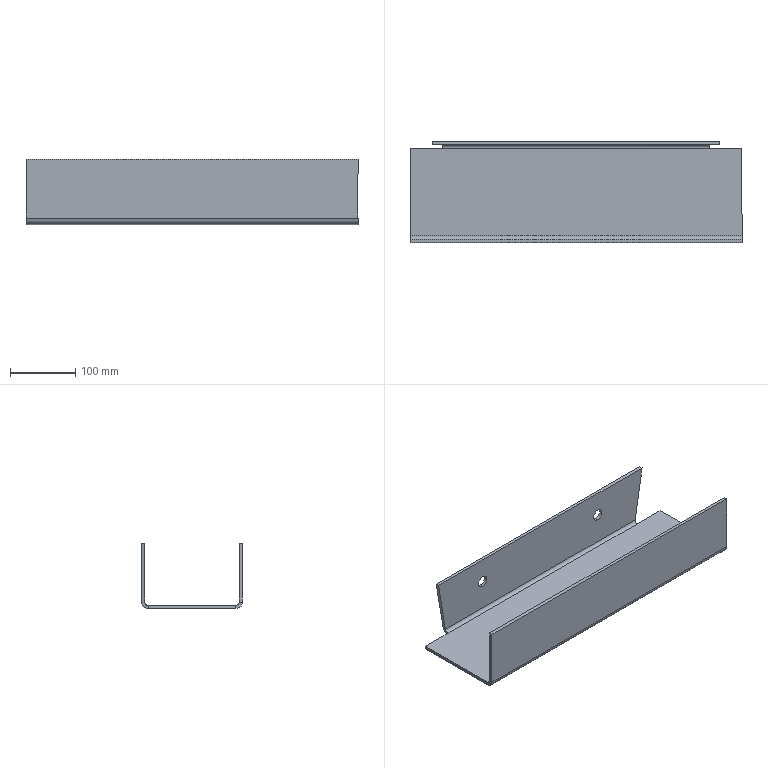Part | SolidWorks | features FlatPattern 1, HoleWzd 1, ICE 1, SM3dBend 1, SMBaseFlange 1, SheetMetal 1, Split 1 | 1 solid | 26 faces | box 510 x 155 x 99.999 mm | volume 817688 mm3 | plane 18 | cylinder 8 | commonest cylinder face diameters 18 x4 10 x2 20 x2
STEP:
#1=CARTESIAN_POINT('',(-125.,72.5,63.414));
#2=VERTEX_POINT('',#1);
#3=CARTESIAN_POINT('',(-125.,72.5,45.414));
#4=VERTEX_POINT('',#3);
#5=CARTESIAN_POINT('',(-125.,72.5,54.414));
#6=DIRECTION('',(0.,-1.,0.));
#7=DIRECTION('',(0.,0.,-1.));
#8=AXIS2_PLACEMENT_3D('',#5,#6,#7);
#9=CIRCLE('',#8,9.);
#10=EDGE_CURVE('',#2,#4,#9,.T.);
#11=ORIENTED_EDGE('',*,*,#10,.T.);
#12=CARTESIAN_POINT('',(-125.,77.5,45.414));
#13=VERTEX_POINT('',#12);
#14=CARTESIAN_POINT('',(-125.,77.5,45.414));
#15=DIRECTION('',(0.,1.,0.));
#16=VECTOR('',#15,1000.);
#17=LINE('',#14,#16);
#18=EDGE_CURVE('',#4,#13,#17,.T.);
#19=ORIENTED_EDGE('',*,*,#18,.T.);
#20=CARTESIAN_POINT('',(-125.,77.5,63.414));
#21=VERTEX_POINT('',#20);
#22=CARTESIAN_POINT('',(-125.,77.5,54.414));
#23=DIRECTION('',(0.,1.,0.));
#24=DIRECTION('',(0.,0.,1.));
#25=AXIS2_PLACEMENT_3D('',#22,#23,#24);
#26=CIRCLE('',#25,9.);
#27=EDGE_CURVE('',#13,#21,#26,.T.);
#28=ORIENTED_EDGE('',*,*,#27,.T.);
#29=CARTESIAN_POINT('',(-125.,77.5,63.414));
#30=DIRECTION('',(0.,1.,0.));
#31=VECTOR('',#30,1000.);
#32=LINE('',#29,#31);
#33=EDGE_CURVE('',#2,#21,#32,.T.);
#34=ORIENTED_EDGE('',*,*,#33,.F.);
#35=EDGE_LOOP('',(#11,#19,#28,#34));
#36=FACE_OUTER_BOUND('',#35,.T.);
#37=CARTESIAN_POINT('',(-125.,77.5,54.414));
#38=DIRECTION('',(0.,1.,0.));
#39=DIRECTION('',(0.,0.,1.));
#40=AXIS2_PLACEMENT_3D('',#37,#38,#39);
#41=CYLINDRICAL_SURFACE('',#40,9.);
#42=ADVANCED_FACE('',(#36),#41,.F.);
#43=CARTESIAN_POINT('',(125.,72.5,63.414));
#44=VERTEX_POINT('',#43);
#45=CARTESIAN_POINT('',(125.,72.5,45.414));
#46=VERTEX_POINT('',#45);
#47=CARTESIAN_POINT('',(125.,72.5,54.414));
#48=DIRECTION('',(0.,-1.,0.));
#49=DIRECTION('',(0.,0.,-1.));
#50=AXIS2_PLACEMENT_3D('',#47,#48,#49);
#51=CIRCLE('',#50,9.);
#52=EDGE_CURVE('',#44,#46,#51,.T.);
#53=ORIENTED_EDGE('',*,*,#52,.T.);
#54=CARTESIAN_POINT('',(125.,77.5,45.414));
#55=VERTEX_POINT('',#54);
#56=CARTESIAN_POINT('',(125.,77.5,45.414));
#57=DIRECTION('',(0.,1.,0.));
#58=VECTOR('',#57,1000.);
#59=LINE('',#56,#58);
#60=EDGE_CURVE('',#46,#55,#59,.T.);
#61=ORIENTED_EDGE('',*,*,#60,.T.);
#62=CARTESIAN_POINT('',(125.,77.5,63.414));
#63=VERTEX_POINT('',#62);
#64=CARTESIAN_POINT('',(125.,77.5,54.414));
#65=DIRECTION('',(0.,1.,0.));
#66=DIRECTION('',(0.,0.,1.));
#67=AXIS2_PLACEMENT_3D('',#64,#65,#66);
#68=CIRCLE('',#67,9.);
#69=EDGE_CURVE('',#55,#63,#68,.T.);
#70=ORIENTED_EDGE('',*,*,#69,.T.);
#71=CARTESIAN_POINT('',(125.,77.5,63.414));
#72=DIRECTION('',(0.,1.,0.));
#73=VECTOR('',#72,1000.);
#74=LINE('',#71,#73);
#75=EDGE_CURVE('',#44,#63,#74,.T.);
#76=ORIENTED_EDGE('',*,*,#75,.F.);
#77=EDGE_LOOP('',(#53,#61,#70,#76));
#78=FACE_OUTER_BOUND('',#77,.T.);
#79=CARTESIAN_POINT('',(125.,77.5,54.414));
#80=DIRECTION('',(0.,1.,0.));
#81=DIRECTION('',(0.,0.,1.));
#82=AXIS2_PLACEMENT_3D('',#79,#80,#81);
#83=CYLINDRICAL_SURFACE('',#82,9.);
#84=ADVANCED_FACE('',(#78),#83,.F.);
#85=CARTESIAN_POINT('',(255.,67.5,0.));
#86=VERTEX_POINT('',#85);
#87=CARTESIAN_POINT('',(205.244,67.5,0.));
#88=VERTEX_POINT('',#87);
#89=CARTESIAN_POINT('',(0.,67.5,0.));
#90=DIRECTION('',(-1.,0.,0.));
#91=VECTOR('',#90,1000.);
#92=LINE('',#89,#91);
#93=EDGE_CURVE('',#86,#88,#92,.T.);
#94=ORIENTED_EDGE('',*,*,#93,.F.);
#95=CARTESIAN_POINT('',(255.,67.5,-5.));
#96=VERTEX_POINT('',#95);
#97=CARTESIAN_POINT('',(255.,67.5,-5.));
#98=DIRECTION('',(0.,0.,-1.));
#99=VECTOR('',#98,1000.);
#100=LINE('',#97,#99);
#101=EDGE_CURVE('',#86,#96,#100,.T.);
#102=ORIENTED_EDGE('',*,*,#101,.T.);
#103=CARTESIAN_POINT('',(204.407,67.5,-5.));
#104=VERTEX_POINT('',#103);
#105=CARTESIAN_POINT('',(0.,67.5,-5.));
#106=DIRECTION('',(-1.,0.,0.));
#107=VECTOR('',#106,1000.);
#108=LINE('',#105,#107);
#109=EDGE_CURVE('',#96,#104,#108,.T.);
#110=ORIENTED_EDGE('',*,*,#109,.T.);
#111=CARTESIAN_POINT('',(199.653,67.5,-33.41));
#112=DIRECTION('',(0.165,0.,0.9863));
#113=VECTOR('',#112,1000.);
#114=LINE('',#111,#113);
#115=EDGE_CURVE('',#104,#88,#114,.T.);
#116=ORIENTED_EDGE('',*,*,#115,.T.);
#117=EDGE_LOOP('',(#94,#102,#110,#116));
#118=FACE_OUTER_BOUND('',#117,.T.);
#119=CARTESIAN_POINT('',(0.,67.5,0.));
#120=DIRECTION('',(0.,1.,0.));
#121=DIRECTION('',(0.,0.,1.));
#122=AXIS2_PLACEMENT_3D('',#119,#120,#121);
#123=PLANE('',#122);
#124=ADVANCED_FACE('',(#118),#123,.T.);
#125=CARTESIAN_POINT('',(-255.,-67.5,-5.));
#126=VERTEX_POINT('',#125);
#127=CARTESIAN_POINT('',(-255.,67.5,-5.));
#128=VERTEX_POINT('',#127);
#129=CARTESIAN_POINT('',(-255.,0.,-5.));
#130=DIRECTION('',(0.,1.,0.));
#131=VECTOR('',#130,1000.);
#132=LINE('',#129,#131);
#133=EDGE_CURVE('',#126,#128,#132,.T.);
#134=ORIENTED_EDGE('',*,*,#133,.T.);
#135=CARTESIAN_POINT('',(-204.437,67.5,-5.));
#136=VERTEX_POINT('',#135);
#137=CARTESIAN_POINT('',(0.,67.5,-5.));
#138=DIRECTION('',(-1.,0.,0.));
#139=VECTOR('',#138,1000.);
#140=LINE('',#137,#139);
#141=EDGE_CURVE('',#136,#128,#140,.T.);
#142=ORIENTED_EDGE('',*,*,#141,.F.);
#143=CARTESIAN_POINT('',(0.,67.5,-5.));
#144=DIRECTION('',(-1.,0.,0.));
#145=VECTOR('',#144,1000.);
#146=LINE('',#143,#145);
#147=EDGE_CURVE('',#104,#136,#146,.T.);
#148=ORIENTED_EDGE('',*,*,#147,.F.);
#149=ORIENTED_EDGE('',*,*,#109,.F.);
#150=CARTESIAN_POINT('',(255.,-67.5,-5.));
#151=VERTEX_POINT('',#150);
#152=CARTESIAN_POINT('',(255.,0.,-5.));
#153=DIRECTION('',(0.,-1.,0.));
#154=VECTOR('',#153,1000.);
#155=LINE('',#152,#154);
#156=EDGE_CURVE('',#96,#151,#155,.T.);
#157=ORIENTED_EDGE('',*,*,#156,.T.);
#158=CARTESIAN_POINT('',(0.,-67.5,-5.));
#159=DIRECTION('',(-1.,0.,0.));
#160=VECTOR('',#159,1000.);
#161=LINE('',#158,#160);
#162=EDGE_CURVE('',#151,#126,#161,.T.);
#163=ORIENTED_EDGE('',*,*,#162,.T.);
#164=EDGE_LOOP('',(#134,#142,#148,#149,#157,#163));
#165=FACE_OUTER_BOUND('',#164,.T.);
#166=CARTESIAN_POINT('',(0.,0.,-5.));
#167=DIRECTION('',(0.,0.,1.));
#168=DIRECTION('',(1.,0.,0.));
#169=AXIS2_PLACEMENT_3D('',#166,#167,#168);
#170=PLANE('',#169);
#171=ADVANCED_FACE('',(#165),#170,.F.);
#172=CARTESIAN_POINT('',(-205.274,67.5,0.));
#173=VERTEX_POINT('',#172);
#174=CARTESIAN_POINT('',(-255.,67.5,0.));
#175=VERTEX_POINT('',#174);
#176=CARTESIAN_POINT('',(0.,67.5,0.));
#177=DIRECTION('',(-1.,0.,0.));
#178=VECTOR('',#177,1000.);
#179=LINE('',#176,#178);
#180=EDGE_CURVE('',#173,#175,#179,.T.);
#181=ORIENTED_EDGE('',*,*,#180,.T.);
#182=CARTESIAN_POINT('',(-255.,-67.5,0.));
#183=VERTEX_POINT('',#182);
#184=CARTESIAN_POINT('',(-255.,0.,0.));
#185=DIRECTION('',(0.,1.,0.));
#186=VECTOR('',#185,1000.);
#187=LINE('',#184,#186);
#188=EDGE_CURVE('',#183,#175,#187,.T.);
#189=ORIENTED_EDGE('',*,*,#188,.F.);
#190=CARTESIAN_POINT('',(255.,-67.5,0.));
#191=VERTEX_POINT('',#190);
#192=CARTESIAN_POINT('',(0.,-67.5,0.));
#193=DIRECTION('',(-1.,0.,0.));
#194=VECTOR('',#193,1000.);
#195=LINE('',#192,#194);
#196=EDGE_CURVE('',#191,#183,#195,.T.);
#197=ORIENTED_EDGE('',*,*,#196,.F.);
#198=CARTESIAN_POINT('',(255.,0.,0.));
#199=DIRECTION('',(0.,-1.,0.));
#200=VECTOR('',#199,1000.);
#201=LINE('',#198,#200);
#202=EDGE_CURVE('',#86,#191,#201,.T.);
#203=ORIENTED_EDGE('',*,*,#202,.F.);
#204=ORIENTED_EDGE('',*,*,#93,.T.);
#205=CARTESIAN_POINT('',(0.,67.5,0.));
#206=DIRECTION('',(-1.,0.,0.));
#207=VECTOR('',#206,1000.);
#208=LINE('',#205,#207);
#209=EDGE_CURVE('',#88,#173,#208,.T.);
#210=ORIENTED_EDGE('',*,*,#209,.T.);
#211=EDGE_LOOP('',(#181,#189,#197,#203,#204,#210));
#212=FACE_OUTER_BOUND('',#211,.T.);
#213=CARTESIAN_POINT('',(0.,0.,0.));
#214=DIRECTION('',(0.,0.,1.));
#215=DIRECTION('',(1.,0.,0.));
#216=AXIS2_PLACEMENT_3D('',#213,#214,#215);
#217=PLANE('',#216);
#218=ADVANCED_FACE('',(#212),#217,.T.);
#219=CARTESIAN_POINT('',(-255.,-72.5,94.999));
#220=VERTEX_POINT('',#219);
#221=CARTESIAN_POINT('',(255.,-72.5,94.999));
#222=VERTEX_POINT('',#221);
#223=CARTESIAN_POINT('',(-275.,-72.5,94.999));
#224=DIRECTION('',(1.,0.,0.));
#225=VECTOR('',#224,1000.);
#226=LINE('',#223,#225);
#227=EDGE_CURVE('',#220,#222,#226,.T.);
#228=ORIENTED_EDGE('',*,*,#227,.F.);
#229=CARTESIAN_POINT('',(-255.,-77.5,94.999));
#230=VERTEX_POINT('',#229);
#231=CARTESIAN_POINT('',(-255.,-77.5,94.999));
#232=DIRECTION('',(0.,-1.,0.));
#233=VECTOR('',#232,1000.);
#234=LINE('',#231,#233);
#235=EDGE_CURVE('',#220,#230,#234,.T.);
#236=ORIENTED_EDGE('',*,*,#235,.T.);
#237=CARTESIAN_POINT('',(255.,-77.5,94.999));
#238=VERTEX_POINT('',#237);
#239=CARTESIAN_POINT('',(-275.,-77.5,94.999));
#240=DIRECTION('',(1.,0.,0.));
#241=VECTOR('',#240,1000.);
#242=LINE('',#239,#241);
#243=EDGE_CURVE('',#230,#238,#242,.T.);
#244=ORIENTED_EDGE('',*,*,#243,.T.);
#245=CARTESIAN_POINT('',(255.,-72.5,94.999));
#246=DIRECTION('',(0.,1.,0.));
#247=VECTOR('',#246,1000.);
#248=LINE('',#245,#247);
#249=EDGE_CURVE('',#238,#222,#248,.T.);
#250=ORIENTED_EDGE('',*,*,#249,.T.);
#251=EDGE_LOOP('',(#228,#236,#244,#250));
#252=FACE_OUTER_BOUND('',#251,.T.);
#253=CARTESIAN_POINT('',(-275.,-77.5,94.999));
#254=DIRECTION('',(0.,0.,1.));
#255=DIRECTION('',(0.,-1.,0.));
#256=AXIS2_PLACEMENT_3D('',#253,#254,#255);
#257=PLANE('',#256);
#258=ADVANCED_FACE('',(#252),#257,.T.);
#259=CARTESIAN_POINT('',(-255.,-72.5,5.));
#260=VERTEX_POINT('',#259);
#261=CARTESIAN_POINT('',(-255.,-67.5,5.));
#262=DIRECTION('',(-1.,0.,0.));
#263=DIRECTION('',(0.,0.,-1.));
#264=AXIS2_PLACEMENT_3D('',#261,#262,#263);
#265=CIRCLE('',#264,5.);
#266=EDGE_CURVE('',#183,#260,#265,.T.);
#267=ORIENTED_EDGE('',*,*,#266,.T.);
#268=CARTESIAN_POINT('',(255.,-72.5,5.));
#269=VERTEX_POINT('',#268);
#270=CARTESIAN_POINT('',(0.,-72.5,5.));
#271=DIRECTION('',(-1.,0.,0.));
#272=VECTOR('',#271,1000.);
#273=LINE('',#270,#272);
#274=EDGE_CURVE('',#269,#260,#273,.T.);
#275=ORIENTED_EDGE('',*,*,#274,.F.);
#276=CARTESIAN_POINT('',(255.,-67.5,5.));
#277=DIRECTION('',(-1.,0.,0.));
#278=DIRECTION('',(0.,0.,-1.));
#279=AXIS2_PLACEMENT_3D('',#276,#277,#278);
#280=CIRCLE('',#279,5.);
#281=EDGE_CURVE('',#191,#269,#280,.T.);
#282=ORIENTED_EDGE('',*,*,#281,.F.);
#283=ORIENTED_EDGE('',*,*,#196,.T.);
#284=EDGE_LOOP('',(#267,#275,#282,#283));
#285=FACE_OUTER_BOUND('',#284,.T.);
#286=CARTESIAN_POINT('',(550.149,-67.5,5.));
#287=DIRECTION('',(-1.,0.,0.));
#288=DIRECTION('',(0.,0.,1.));
#289=AXIS2_PLACEMENT_3D('',#286,#287,#288);
#290=CYLINDRICAL_SURFACE('',#289,5.);
#291=ADVANCED_FACE('',(#285),#290,.F.);
#292=ORIENTED_EDGE('',*,*,#274,.T.);
#293=CARTESIAN_POINT('',(-255.,-72.5,50.));
#294=DIRECTION('',(0.,0.,-1.));
#295=VECTOR('',#294,1000.);
#296=LINE('',#293,#295);
#297=EDGE_CURVE('',#220,#260,#296,.T.);
#298=ORIENTED_EDGE('',*,*,#297,.F.);
#299=ORIENTED_EDGE('',*,*,#227,.T.);
#300=CARTESIAN_POINT('',(255.,-72.5,-74.281));
#301=DIRECTION('',(0.,0.,-1.));
#302=VECTOR('',#301,1000.);
#303=LINE('',#300,#302);
#304=EDGE_CURVE('',#222,#269,#303,.T.);
#305=ORIENTED_EDGE('',*,*,#304,.T.);
#306=EDGE_LOOP('',(#292,#298,#299,#305));
#307=FACE_OUTER_BOUND('',#306,.T.);
#308=CARTESIAN_POINT('',(0.,-72.5,-74.281));
#309=DIRECTION('',(0.,1.,0.));
#310=DIRECTION('',(1.,0.,0.));
#311=AXIS2_PLACEMENT_3D('',#308,#309,#310);
#312=PLANE('',#311);
#313=ADVANCED_FACE('',(#307),#312,.T.);
#314=CARTESIAN_POINT('',(255.,-77.5,5.));
#315=VERTEX_POINT('',#314);
#316=CARTESIAN_POINT('',(-255.,-77.5,5.));
#317=VERTEX_POINT('',#316);
#318=CARTESIAN_POINT('',(0.,-77.5,5.));
#319=DIRECTION('',(-1.,0.,0.));
#320=VECTOR('',#319,1000.);
#321=LINE('',#318,#320);
#322=EDGE_CURVE('',#315,#317,#321,.T.);
#323=ORIENTED_EDGE('',*,*,#322,.T.);
#324=CARTESIAN_POINT('',(-255.,-67.5,5.));
#325=DIRECTION('',(-1.,0.,0.));
#326=DIRECTION('',(0.,0.,1.));
#327=AXIS2_PLACEMENT_3D('',#324,#325,#326);
#328=CIRCLE('',#327,10.);
#329=EDGE_CURVE('',#126,#317,#328,.T.);
#330=ORIENTED_EDGE('',*,*,#329,.F.);
#331=ORIENTED_EDGE('',*,*,#162,.F.);
#332=CARTESIAN_POINT('',(255.,-67.5,5.));
#333=DIRECTION('',(-1.,0.,0.));
#334=DIRECTION('',(0.,0.,1.));
#335=AXIS2_PLACEMENT_3D('',#332,#333,#334);
#336=CIRCLE('',#335,10.);
#337=EDGE_CURVE('',#151,#315,#336,.T.);
#338=ORIENTED_EDGE('',*,*,#337,.T.);
#339=EDGE_LOOP('',(#323,#330,#331,#338));
#340=FACE_OUTER_BOUND('',#339,.T.);
#341=CARTESIAN_POINT('',(550.149,-67.5,5.));
#342=DIRECTION('',(-1.,0.,0.));
#343=DIRECTION('',(0.,0.,1.));
#344=AXIS2_PLACEMENT_3D('',#341,#342,#343);
#345=CYLINDRICAL_SURFACE('',#344,10.);
#346=ADVANCED_FACE('',(#340),#345,.T.);
#347=CARTESIAN_POINT('',(-255.,-77.5,-74.281));
#348=DIRECTION('',(0.,0.,-1.));
#349=VECTOR('',#348,1000.);
#350=LINE('',#347,#349);
#351=EDGE_CURVE('',#230,#317,#350,.T.);
#352=ORIENTED_EDGE('',*,*,#351,.T.);
#353=ORIENTED_EDGE('',*,*,#322,.F.);
#354=CARTESIAN_POINT('',(255.,-77.5,50.));
#355=DIRECTION('',(0.,0.,-1.));
#356=VECTOR('',#355,1000.);
#357=LINE('',#354,#356);
#358=EDGE_CURVE('',#238,#315,#357,.T.);
#359=ORIENTED_EDGE('',*,*,#358,.F.);
#360=ORIENTED_EDGE('',*,*,#243,.F.);
#361=EDGE_LOOP('',(#352,#353,#359,#360));
#362=FACE_OUTER_BOUND('',#361,.T.);
#363=CARTESIAN_POINT('',(0.,-77.5,-74.281));
#364=DIRECTION('',(0.,1.,0.));
#365=DIRECTION('',(1.,0.,0.));
#366=AXIS2_PLACEMENT_3D('',#363,#364,#365);
#367=PLANE('',#366);
#368=ADVANCED_FACE('',(#362),#367,.F.);
#369=ORIENTED_EDGE('',*,*,#141,.T.);
#370=CARTESIAN_POINT('',(-255.,67.5,-5.));
#371=DIRECTION('',(0.,0.,-1.));
#372=VECTOR('',#371,1000.);
#373=LINE('',#370,#372);
#374=EDGE_CURVE('',#175,#128,#373,.T.);
#375=ORIENTED_EDGE('',*,*,#374,.F.);
#376=ORIENTED_EDGE('',*,*,#180,.F.);
#377=CARTESIAN_POINT('',(-199.682,67.5,-33.415));
#378=DIRECTION('',(0.165,0.,-0.9863));
#379=VECTOR('',#378,1000.);
#380=LINE('',#377,#379);
#381=EDGE_CURVE('',#173,#136,#380,.T.);
#382=ORIENTED_EDGE('',*,*,#381,.T.);
#383=EDGE_LOOP('',(#369,#375,#376,#382));
#384=FACE_OUTER_BOUND('',#383,.T.);
#385=CARTESIAN_POINT('',(0.,67.5,0.));
#386=DIRECTION('',(0.,1.,0.));
#387=DIRECTION('',(0.,0.,1.));
#388=AXIS2_PLACEMENT_3D('',#385,#386,#387);
#389=PLANE('',#388);
#390=ADVANCED_FACE('',(#384),#389,.T.);
#391=ORIENTED_EDGE('',*,*,#115,.F.);
#392=CARTESIAN_POINT('',(206.08,77.5,5.));
#393=VERTEX_POINT('',#392);
#394=CARTESIAN_POINT('',(204.407,67.5,-5.));
#395=CARTESIAN_POINT('',(204.407,73.358,-5.));
#396=CARTESIAN_POINT('',(205.1,77.5,-0.8579));
#397=CARTESIAN_POINT('',(206.08,77.5,5.));
#398=(BOUNDED_CURVE()B_SPLINE_CURVE(3,(#394,#395,#396,#397),.UNSPECIFIED.,.F.,.T.)B_SPLINE_CURVE_WITH_KNOTS((4,4),(3.142,4.712),.UNSPECIFIED.)CURVE()GEOMETRIC_REPRESENTATION_ITEM()RATIONAL_B_SPLINE_CURVE((1.,0.8047,0.8047,1.))REPRESENTATION_ITEM(''));
#399=EDGE_CURVE('',#104,#393,#398,.T.);
#400=ORIENTED_EDGE('',*,*,#399,.T.);
#401=CARTESIAN_POINT('',(221.141,77.5,94.999));
#402=VERTEX_POINT('',#401);
#403=CARTESIAN_POINT('',(187.561,77.5,-105.668));
#404=DIRECTION('',(-0.165,0.,-0.9863));
#405=VECTOR('',#404,1000.);
#406=LINE('',#403,#405);
#407=EDGE_CURVE('',#402,#393,#406,.T.);
#408=ORIENTED_EDGE('',*,*,#407,.F.);
#409=CARTESIAN_POINT('',(221.141,72.5,94.999));
#410=VERTEX_POINT('',#409);
#411=CARTESIAN_POINT('',(221.141,77.5,94.999));
#412=DIRECTION('',(0.,-1.,0.));
#413=VECTOR('',#412,1000.);
#414=LINE('',#411,#413);
#415=EDGE_CURVE('',#402,#410,#414,.T.);
#416=ORIENTED_EDGE('',*,*,#415,.T.);
#417=CARTESIAN_POINT('',(206.08,72.5,5.));
#418=VERTEX_POINT('',#417);
#419=CARTESIAN_POINT('',(187.561,72.5,-105.668));
#420=DIRECTION('',(-0.165,0.,-0.9863));
#421=VECTOR('',#420,1000.);
#422=LINE('',#419,#421);
#423=EDGE_CURVE('',#410,#418,#422,.T.);
#424=ORIENTED_EDGE('',*,*,#423,.T.);
#425=CARTESIAN_POINT('',(205.244,67.5,0.));
#426=CARTESIAN_POINT('',(205.244,70.429,0.));
#427=CARTESIAN_POINT('',(205.59,72.5,2.071));
#428=CARTESIAN_POINT('',(206.08,72.5,5.));
#429=(BOUNDED_CURVE()B_SPLINE_CURVE(3,(#425,#426,#427,#428),.UNSPECIFIED.,.F.,.T.)B_SPLINE_CURVE_WITH_KNOTS((4,4),(3.142,4.712),.UNSPECIFIED.)CURVE()GEOMETRIC_REPRESENTATION_ITEM()RATIONAL_B_SPLINE_CURVE((1.,0.8047,0.8047,1.))REPRESENTATION_ITEM(''));
#430=EDGE_CURVE('',#88,#418,#429,.T.);
#431=ORIENTED_EDGE('',*,*,#430,.F.);
#432=EDGE_LOOP('',(#391,#400,#408,#416,#424,#431));
#433=FACE_OUTER_BOUND('',#432,.T.);
#434=CARTESIAN_POINT('',(199.653,0.,-33.41));
#435=DIRECTION('',(-0.9863,0.,0.165));
#436=DIRECTION('',(0.165,0.,0.9863));
#437=AXIS2_PLACEMENT_3D('',#434,#435,#436);
#438=PLANE('',#437);
#439=ADVANCED_FACE('',(#433),#438,.F.);
#440=CARTESIAN_POINT('',(-206.11,77.5,5.));
#441=VERTEX_POINT('',#440);
#442=CARTESIAN_POINT('',(-206.11,77.5,5.));
#443=CARTESIAN_POINT('',(-205.13,77.5,-0.8579));
#444=CARTESIAN_POINT('',(-204.437,73.358,-5.));
#445=CARTESIAN_POINT('',(-204.437,67.5,-5.));
#446=(BOUNDED_CURVE()B_SPLINE_CURVE(3,(#442,#443,#444,#445),.UNSPECIFIED.,.F.,.T.)B_SPLINE_CURVE_WITH_KNOTS((4,4),(4.712,6.283),.UNSPECIFIED.)CURVE()GEOMETRIC_REPRESENTATION_ITEM()RATIONAL_B_SPLINE_CURVE((1.,0.8047,0.8047,1.))REPRESENTATION_ITEM(''));
#447=EDGE_CURVE('',#441,#136,#446,.T.);
#448=ORIENTED_EDGE('',*,*,#447,.T.);
#449=ORIENTED_EDGE('',*,*,#381,.F.);
#450=CARTESIAN_POINT('',(-206.11,72.5,5.));
#451=VERTEX_POINT('',#450);
#452=CARTESIAN_POINT('',(-206.11,72.5,5.));
#453=CARTESIAN_POINT('',(-205.62,72.5,2.071));
#454=CARTESIAN_POINT('',(-205.274,70.429,0.));
#455=CARTESIAN_POINT('',(-205.274,67.5,0.));
#456=(BOUNDED_CURVE()B_SPLINE_CURVE(3,(#452,#453,#454,#455),.UNSPECIFIED.,.F.,.T.)B_SPLINE_CURVE_WITH_KNOTS((4,4),(4.712,6.283),.UNSPECIFIED.)CURVE()GEOMETRIC_REPRESENTATION_ITEM()RATIONAL_B_SPLINE_CURVE((1.,0.8047,0.8047,1.))REPRESENTATION_ITEM(''));
#457=EDGE_CURVE('',#451,#173,#456,.T.);
#458=ORIENTED_EDGE('',*,*,#457,.F.);
#459=CARTESIAN_POINT('',(-221.171,72.5,94.999));
#460=VERTEX_POINT('',#459);
#461=CARTESIAN_POINT('',(-187.59,72.5,-105.673));
#462=DIRECTION('',(-0.165,0.,0.9863));
#463=VECTOR('',#462,1000.);
#464=LINE('',#461,#463);
#465=EDGE_CURVE('',#451,#460,#464,.T.);
#466=ORIENTED_EDGE('',*,*,#465,.T.);
#467=CARTESIAN_POINT('',(-221.171,77.5,94.999));
#468=VERTEX_POINT('',#467);
#469=CARTESIAN_POINT('',(-221.171,77.5,94.999));
#470=DIRECTION('',(0.,1.,0.));
#471=VECTOR('',#470,1000.);
#472=LINE('',#469,#471);
#473=EDGE_CURVE('',#460,#468,#472,.T.);
#474=ORIENTED_EDGE('',*,*,#473,.T.);
#475=CARTESIAN_POINT('',(-187.59,77.5,-105.673));
#476=DIRECTION('',(-0.165,0.,0.9863));
#477=VECTOR('',#476,1000.);
#478=LINE('',#475,#477);
#479=EDGE_CURVE('',#441,#468,#478,.T.);
#480=ORIENTED_EDGE('',*,*,#479,.F.);
#481=EDGE_LOOP('',(#448,#449,#458,#466,#474,#480));
#482=FACE_OUTER_BOUND('',#481,.T.);
#483=CARTESIAN_POINT('',(-199.682,0.,-33.415));
#484=DIRECTION('',(0.9863,0.,0.165));
#485=DIRECTION('',(0.165,0.,-0.9863));
#486=AXIS2_PLACEMENT_3D('',#483,#484,#485);
#487=PLANE('',#486);
#488=ADVANCED_FACE('',(#482),#487,.F.);
#489=CARTESIAN_POINT('',(-125.,77.5,54.414));
#490=DIRECTION('',(0.,1.,0.));
#491=DIRECTION('',(0.,0.,1.));
#492=AXIS2_PLACEMENT_3D('',#489,#490,#491);
#493=CIRCLE('',#492,9.);
#494=EDGE_CURVE('',#21,#13,#493,.T.);
#495=ORIENTED_EDGE('',*,*,#494,.F.);
#496=ORIENTED_EDGE('',*,*,#27,.F.);
#497=EDGE_LOOP('',(#495,#496));
#498=FACE_BOUND('',#497,.T.);
#499=CARTESIAN_POINT('',(125.,77.5,54.414));
#500=DIRECTION('',(0.,1.,0.));
#501=DIRECTION('',(0.,0.,1.));
#502=AXIS2_PLACEMENT_3D('',#499,#500,#501);
#503=CIRCLE('',#502,9.);
#504=EDGE_CURVE('',#63,#55,#503,.T.);
#505=ORIENTED_EDGE('',*,*,#504,.F.);
#506=ORIENTED_EDGE('',*,*,#69,.F.);
#507=EDGE_LOOP('',(#505,#506));
#508=FACE_BOUND('',#507,.T.);
#509=CARTESIAN_POINT('',(-275.,77.5,94.999));
#510=DIRECTION('',(-1.,0.,0.));
#511=VECTOR('',#510,1000.);
#512=LINE('',#509,#511);
#513=EDGE_CURVE('',#402,#468,#512,.T.);
#514=ORIENTED_EDGE('',*,*,#513,.F.);
#515=ORIENTED_EDGE('',*,*,#407,.T.);
#516=CARTESIAN_POINT('',(0.,77.5,5.));
#517=DIRECTION('',(-1.,0.,0.));
#518=VECTOR('',#517,1000.);
#519=LINE('',#516,#518);
#520=EDGE_CURVE('',#393,#441,#519,.T.);
#521=ORIENTED_EDGE('',*,*,#520,.T.);
#522=ORIENTED_EDGE('',*,*,#479,.T.);
#523=EDGE_LOOP('',(#514,#515,#521,#522));
#524=FACE_OUTER_BOUND('',#523,.T.);
#525=CARTESIAN_POINT('',(0.,77.5,-74.281));
#526=DIRECTION('',(0.,-1.,0.));
#527=DIRECTION('',(1.,0.,0.));
#528=AXIS2_PLACEMENT_3D('',#525,#526,#527);
#529=PLANE('',#528);
#530=ADVANCED_FACE('',(#498,#508,#524),#529,.F.);
#531=ORIENTED_EDGE('',*,*,#10,.F.);
#532=CARTESIAN_POINT('',(-125.,72.5,54.414));
#533=DIRECTION('',(0.,-1.,0.));
#534=DIRECTION('',(0.,0.,-1.));
#535=AXIS2_PLACEMENT_3D('',#532,#533,#534);
#536=CIRCLE('',#535,9.);
#537=EDGE_CURVE('',#4,#2,#536,.T.);
#538=ORIENTED_EDGE('',*,*,#537,.F.);
#539=EDGE_LOOP('',(#531,#538));
#540=FACE_BOUND('',#539,.T.);
#541=ORIENTED_EDGE('',*,*,#52,.F.);
#542=CARTESIAN_POINT('',(125.,72.5,54.414));
#543=DIRECTION('',(0.,-1.,0.));
#544=DIRECTION('',(0.,0.,-1.));
#545=AXIS2_PLACEMENT_3D('',#542,#543,#544);
#546=CIRCLE('',#545,9.);
#547=EDGE_CURVE('',#46,#44,#546,.T.);
#548=ORIENTED_EDGE('',*,*,#547,.F.);
#549=EDGE_LOOP('',(#541,#548));
#550=FACE_BOUND('',#549,.T.);
#551=ORIENTED_EDGE('',*,*,#423,.F.);
#552=CARTESIAN_POINT('',(-275.,72.5,94.999));
#553=DIRECTION('',(-1.,0.,0.));
#554=VECTOR('',#553,1000.);
#555=LINE('',#552,#554);
#556=EDGE_CURVE('',#410,#460,#555,.T.);
#557=ORIENTED_EDGE('',*,*,#556,.T.);
#558=ORIENTED_EDGE('',*,*,#465,.F.);
#559=CARTESIAN_POINT('',(0.,72.5,5.));
#560=DIRECTION('',(-1.,0.,0.));
#561=VECTOR('',#560,1000.);
#562=LINE('',#559,#561);
#563=EDGE_CURVE('',#418,#451,#562,.T.);
#564=ORIENTED_EDGE('',*,*,#563,.F.);
#565=EDGE_LOOP('',(#551,#557,#558,#564));
#566=FACE_OUTER_BOUND('',#565,.T.);
#567=CARTESIAN_POINT('',(0.,72.5,-74.281));
#568=DIRECTION('',(0.,-1.,0.));
#569=DIRECTION('',(1.,0.,0.));
#570=AXIS2_PLACEMENT_3D('',#567,#568,#569);
#571=PLANE('',#570);
#572=ADVANCED_FACE('',(#540,#550,#566),#571,.T.);
#573=ORIENTED_EDGE('',*,*,#415,.F.);
#574=ORIENTED_EDGE('',*,*,#513,.T.);
#575=ORIENTED_EDGE('',*,*,#473,.F.);
#576=ORIENTED_EDGE('',*,*,#556,.F.);
#577=EDGE_LOOP('',(#573,#574,#575,#576));
#578=FACE_OUTER_BOUND('',#577,.T.);
#579=CARTESIAN_POINT('',(-275.,77.5,94.999));
#580=DIRECTION('',(0.,0.,1.));
#581=DIRECTION('',(0.,-1.,0.));
#582=AXIS2_PLACEMENT_3D('',#579,#580,#581);
#583=PLANE('',#582);
#584=ADVANCED_FACE('',(#578),#583,.T.);
#585=ORIENTED_EDGE('',*,*,#209,.F.);
#586=ORIENTED_EDGE('',*,*,#430,.T.);
#587=ORIENTED_EDGE('',*,*,#563,.T.);
#588=ORIENTED_EDGE('',*,*,#457,.T.);
#589=EDGE_LOOP('',(#585,#586,#587,#588));
#590=FACE_OUTER_BOUND('',#589,.T.);
#591=CARTESIAN_POINT('',(-550.149,67.5,5.));
#592=DIRECTION('',(1.,0.,0.));
#593=DIRECTION('',(0.,0.,-1.));
#594=AXIS2_PLACEMENT_3D('',#591,#592,#593);
#595=CYLINDRICAL_SURFACE('',#594,5.);
#596=ADVANCED_FACE('',(#590),#595,.F.);
#597=ORIENTED_EDGE('',*,*,#399,.F.);
#598=ORIENTED_EDGE('',*,*,#147,.T.);
#599=ORIENTED_EDGE('',*,*,#447,.F.);
#600=ORIENTED_EDGE('',*,*,#520,.F.);
#601=EDGE_LOOP('',(#597,#598,#599,#600));
#602=FACE_OUTER_BOUND('',#601,.T.);
#603=CARTESIAN_POINT('',(-550.149,67.5,5.));
#604=DIRECTION('',(1.,0.,0.));
#605=DIRECTION('',(0.,0.,-1.));
#606=AXIS2_PLACEMENT_3D('',#603,#604,#605);
#607=CYLINDRICAL_SURFACE('',#606,10.);
#608=ADVANCED_FACE('',(#602),#607,.T.);
#609=ORIENTED_EDGE('',*,*,#60,.F.);
#610=ORIENTED_EDGE('',*,*,#547,.T.);
#611=ORIENTED_EDGE('',*,*,#75,.T.);
#612=ORIENTED_EDGE('',*,*,#504,.T.);
#613=EDGE_LOOP('',(#609,#610,#611,#612));
#614=FACE_OUTER_BOUND('',#613,.T.);
#615=CARTESIAN_POINT('',(125.,77.5,54.414));
#616=DIRECTION('',(0.,1.,0.));
#617=DIRECTION('',(0.,0.,1.));
#618=AXIS2_PLACEMENT_3D('',#615,#616,#617);
#619=CYLINDRICAL_SURFACE('',#618,9.);
#620=ADVANCED_FACE('',(#614),#619,.F.);
#621=ORIENTED_EDGE('',*,*,#18,.F.);
#622=ORIENTED_EDGE('',*,*,#537,.T.);
#623=ORIENTED_EDGE('',*,*,#33,.T.);
#624=ORIENTED_EDGE('',*,*,#494,.T.);
#625=EDGE_LOOP('',(#621,#622,#623,#624));
#626=FACE_OUTER_BOUND('',#625,.T.);
#627=CARTESIAN_POINT('',(-125.,77.5,54.414));
#628=DIRECTION('',(0.,1.,0.));
#629=DIRECTION('',(0.,0.,1.));
#630=AXIS2_PLACEMENT_3D('',#627,#628,#629);
#631=CYLINDRICAL_SURFACE('',#630,9.);
#632=ADVANCED_FACE('',(#626),#631,.F.);
#633=ORIENTED_EDGE('',*,*,#188,.T.);
#634=ORIENTED_EDGE('',*,*,#374,.T.);
#635=ORIENTED_EDGE('',*,*,#133,.F.);
#636=CARTESIAN_POINT('',(-255.,-67.5,0.));
#637=DIRECTION('',(0.,0.,-1.));
#638=VECTOR('',#637,1000.);
#639=LINE('',#636,#638);
#640=EDGE_CURVE('',#183,#126,#639,.T.);
#641=ORIENTED_EDGE('',*,*,#640,.F.);
#642=EDGE_LOOP('',(#633,#634,#635,#641));
#643=FACE_OUTER_BOUND('',#642,.T.);
#644=CARTESIAN_POINT('',(-255.,0.,-5.));
#645=DIRECTION('',(1.,0.,0.));
#646=DIRECTION('',(0.,1.,0.));
#647=AXIS2_PLACEMENT_3D('',#644,#645,#646);
#648=PLANE('',#647);
#649=ADVANCED_FACE('',(#643),#648,.F.);
#650=CARTESIAN_POINT('',(-255.,-72.5,5.));
#651=DIRECTION('',(0.,-1.,0.));
#652=VECTOR('',#651,1000.);
#653=LINE('',#650,#652);
#654=EDGE_CURVE('',#260,#317,#653,.T.);
#655=ORIENTED_EDGE('',*,*,#654,.F.);
#656=ORIENTED_EDGE('',*,*,#266,.F.);
#657=ORIENTED_EDGE('',*,*,#640,.T.);
#658=ORIENTED_EDGE('',*,*,#329,.T.);
#659=EDGE_LOOP('',(#655,#656,#657,#658));
#660=FACE_OUTER_BOUND('',#659,.T.);
#661=CARTESIAN_POINT('',(-255.,-67.5,5.));
#662=DIRECTION('',(-1.,0.,0.));
#663=DIRECTION('',(0.,0.,1.));
#664=AXIS2_PLACEMENT_3D('',#661,#662,#663);
#665=PLANE('',#664);
#666=ADVANCED_FACE('',(#660),#665,.T.);
#667=ORIENTED_EDGE('',*,*,#297,.T.);
#668=ORIENTED_EDGE('',*,*,#654,.T.);
#669=ORIENTED_EDGE('',*,*,#351,.F.);
#670=ORIENTED_EDGE('',*,*,#235,.F.);
#671=EDGE_LOOP('',(#667,#668,#669,#670));
#672=FACE_OUTER_BOUND('',#671,.T.);
#673=CARTESIAN_POINT('',(-255.,-77.5,-74.281));
#674=DIRECTION('',(1.,0.,0.));
#675=DIRECTION('',(0.,0.,-1.));
#676=AXIS2_PLACEMENT_3D('',#673,#674,#675);
#677=PLANE('',#676);
#678=ADVANCED_FACE('',(#672),#677,.F.);
#679=ORIENTED_EDGE('',*,*,#281,.T.);
#680=CARTESIAN_POINT('',(255.,-77.5,5.));
#681=DIRECTION('',(0.,1.,0.));
#682=VECTOR('',#681,1000.);
#683=LINE('',#680,#682);
#684=EDGE_CURVE('',#315,#269,#683,.T.);
#685=ORIENTED_EDGE('',*,*,#684,.F.);
#686=ORIENTED_EDGE('',*,*,#337,.F.);
#687=CARTESIAN_POINT('',(255.,-67.5,-5.));
#688=DIRECTION('',(0.,0.,1.));
#689=VECTOR('',#688,1000.);
#690=LINE('',#687,#689);
#691=EDGE_CURVE('',#151,#191,#690,.T.);
#692=ORIENTED_EDGE('',*,*,#691,.T.);
#693=EDGE_LOOP('',(#679,#685,#686,#692));
#694=FACE_OUTER_BOUND('',#693,.T.);
#695=CARTESIAN_POINT('',(255.,-67.5,5.));
#696=DIRECTION('',(1.,0.,0.));
#697=DIRECTION('',(0.,0.,-1.));
#698=AXIS2_PLACEMENT_3D('',#695,#696,#697);
#699=PLANE('',#698);
#700=ADVANCED_FACE('',(#694),#699,.T.);
#701=ORIENTED_EDGE('',*,*,#101,.F.);
#702=ORIENTED_EDGE('',*,*,#202,.T.);
#703=ORIENTED_EDGE('',*,*,#691,.F.);
#704=ORIENTED_EDGE('',*,*,#156,.F.);
#705=EDGE_LOOP('',(#701,#702,#703,#704));
#706=FACE_OUTER_BOUND('',#705,.T.);
#707=CARTESIAN_POINT('',(255.,0.,-5.));
#708=DIRECTION('',(-1.,0.,0.));
#709=DIRECTION('',(0.,-1.,0.));
#710=AXIS2_PLACEMENT_3D('',#707,#708,#709);
#711=PLANE('',#710);
#712=ADVANCED_FACE('',(#706),#711,.F.);
#713=ORIENTED_EDGE('',*,*,#249,.F.);
#714=ORIENTED_EDGE('',*,*,#358,.T.);
#715=ORIENTED_EDGE('',*,*,#684,.T.);
#716=ORIENTED_EDGE('',*,*,#304,.F.);
#717=EDGE_LOOP('',(#713,#714,#715,#716));
#718=FACE_OUTER_BOUND('',#717,.T.);
#719=CARTESIAN_POINT('',(255.,-72.5,-74.281));
#720=DIRECTION('',(-1.,0.,0.));
#721=DIRECTION('',(0.,0.,-1.));
#722=AXIS2_PLACEMENT_3D('',#719,#720,#721);
#723=PLANE('',#722);
#724=ADVANCED_FACE('',(#718),#723,.F.);
#725=CLOSED_SHELL('',(#42,#84,#124,#171,#218,#258,#291,#313,#346,#368,#390,#439,#488,#530,#572,#584,#596,#608,#620,#632,#649,#666,#678,#700,#712,#724));
#726=MANIFOLD_SOLID_BREP('',#725);
#727=CARTESIAN_POINT('',(0.,0.,0.));
#728=DIRECTION('',(0.,0.,1.));
#729=DIRECTION('',(1.,0.,0.));
#730=AXIS2_PLACEMENT_3D('',#727,#728,#729);
#731=(LENGTH_UNIT()NAMED_UNIT(*)SI_UNIT(.MILLI.,.METRE.));
#732=UNCERTAINTY_MEASURE_WITH_UNIT(LENGTH_MEASURE(0.00001),#731,'','');
#733=(NAMED_UNIT(*)PLANE_ANGLE_UNIT()SI_UNIT($,.RADIAN.));
#734=(NAMED_UNIT(*)SI_UNIT($,.STERADIAN.)SOLID_ANGLE_UNIT());
#735=(GEOMETRIC_REPRESENTATION_CONTEXT(3)GLOBAL_UNCERTAINTY_ASSIGNED_CONTEXT((#732))GLOBAL_UNIT_ASSIGNED_CONTEXT((#731,#733,#734))REPRESENTATION_CONTEXT('',''));
#736=ADVANCED_BREP_SHAPE_REPRESENTATION('',(#726,#730),#735);